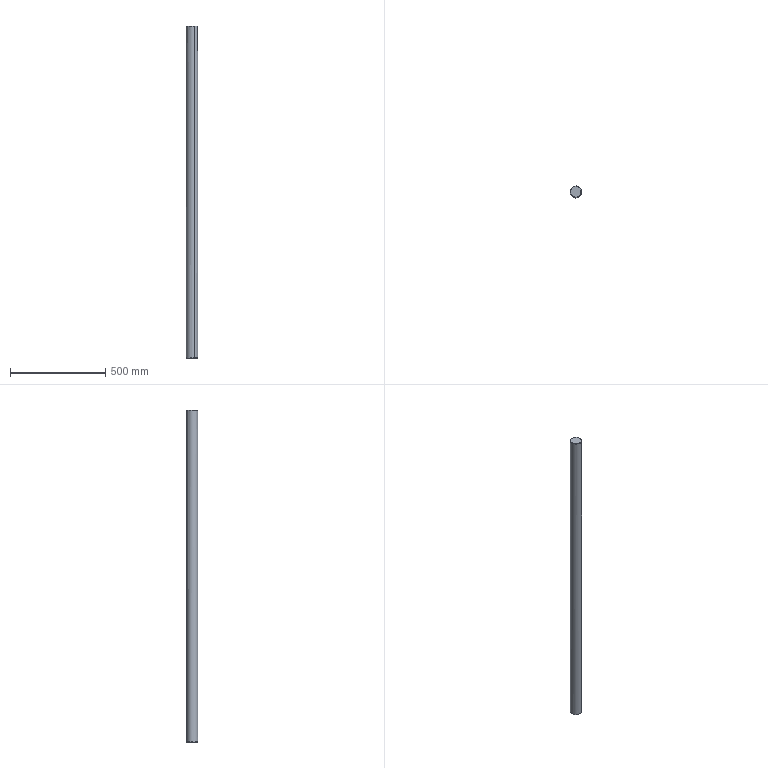Part | SolidWorks | features BaseBody 1 | 1 solid | 16 faces | box 60 x 60 x 1739 mm | volume 4902443 mm3 | cone 6 | plane 5 | cylinder 5 | commonest cylinder face diameters 18 x3 60 x2
STEP:
#1=CARTESIAN_POINT('',(-163.923,853.249,-864.893));
#2=VERTEX_POINT('',#1);
#3=CARTESIAN_POINT('',(-161.923,853.249,-862.893));
#4=VERTEX_POINT('',#3);
#5=CARTESIAN_POINT('',(-161.923,853.249,-862.893));
#6=DIRECTION('',(0.7071,0.,0.7071));
#7=VECTOR('',#6,1000.);
#8=LINE('',#5,#7);
#9=EDGE_CURVE('',#2,#4,#8,.T.);
#10=ORIENTED_EDGE('',*,*,#9,.F.);
#11=CARTESIAN_POINT('',(-203.98,878.52,-864.893));
#12=VERTEX_POINT('',#11);
#13=CARTESIAN_POINT('',(-191.923,853.249,-864.893));
#14=DIRECTION('',(0.,0.,-1.));
#15=DIRECTION('',(-1.,0.,0.));
#16=AXIS2_PLACEMENT_3D('',#13,#14,#15);
#17=CIRCLE('',#16,28.);
#18=EDGE_CURVE('',#12,#2,#17,.T.);
#19=ORIENTED_EDGE('',*,*,#18,.F.);
#20=CARTESIAN_POINT('',(-204.841,880.325,-862.893));
#21=VERTEX_POINT('',#20);
#22=CARTESIAN_POINT('',(-203.98,878.52,-864.893));
#23=DIRECTION('',(-0.3045,0.6382,0.7071));
#24=VECTOR('',#23,1000.);
#25=LINE('',#22,#24);
#26=EDGE_CURVE('',#12,#21,#25,.T.);
#27=ORIENTED_EDGE('',*,*,#26,.T.);
#28=CARTESIAN_POINT('',(-191.923,853.249,-862.893));
#29=DIRECTION('',(0.,0.,1.));
#30=DIRECTION('',(-1.,0.,0.));
#31=AXIS2_PLACEMENT_3D('',#28,#29,#30);
#32=CIRCLE('',#31,30.);
#33=EDGE_CURVE('',#4,#21,#32,.T.);
#34=ORIENTED_EDGE('',*,*,#33,.F.);
#35=EDGE_LOOP('',(#10,#19,#27,#34));
#36=FACE_OUTER_BOUND('',#35,.T.);
#37=CARTESIAN_POINT('',(-191.923,853.249,-862.893));
#38=DIRECTION('',(0.,0.,1.));
#39=DIRECTION('',(1.,0.,0.));
#40=AXIS2_PLACEMENT_3D('',#37,#38,#39);
#41=CONICAL_SURFACE('',#40,30.,0.7854);
#42=ADVANCED_FACE('',(#36),#41,.T.);
#43=ORIENTED_EDGE('',*,*,#26,.F.);
#44=CARTESIAN_POINT('',(-179.866,827.978,-864.893));
#45=VERTEX_POINT('',#44);
#46=CARTESIAN_POINT('',(-191.923,853.249,-864.893));
#47=DIRECTION('',(0.,0.,-1.));
#48=DIRECTION('',(-1.,0.,0.));
#49=AXIS2_PLACEMENT_3D('',#46,#47,#48);
#50=CIRCLE('',#49,28.);
#51=EDGE_CURVE('',#45,#12,#50,.T.);
#52=ORIENTED_EDGE('',*,*,#51,.F.);
#53=CARTESIAN_POINT('',(-179.005,826.173,-862.893));
#54=VERTEX_POINT('',#53);
#55=CARTESIAN_POINT('',(-179.005,826.173,-862.893));
#56=DIRECTION('',(-0.3045,0.6382,-0.7071));
#57=VECTOR('',#56,1000.);
#58=LINE('',#55,#57);
#59=EDGE_CURVE('',#54,#45,#58,.T.);
#60=ORIENTED_EDGE('',*,*,#59,.F.);
#61=CARTESIAN_POINT('',(-191.923,853.249,-862.893));
#62=DIRECTION('',(0.,0.,1.));
#63=DIRECTION('',(-1.,0.,0.));
#64=AXIS2_PLACEMENT_3D('',#61,#62,#63);
#65=CIRCLE('',#64,30.);
#66=EDGE_CURVE('',#21,#54,#65,.T.);
#67=ORIENTED_EDGE('',*,*,#66,.F.);
#68=EDGE_LOOP('',(#43,#52,#60,#67));
#69=FACE_OUTER_BOUND('',#68,.T.);
#70=CARTESIAN_POINT('',(-191.923,853.249,-862.893));
#71=DIRECTION('',(0.,0.,1.));
#72=DIRECTION('',(1.,0.,0.));
#73=AXIS2_PLACEMENT_3D('',#70,#71,#72);
#74=CONICAL_SURFACE('',#73,30.,0.7854);
#75=ADVANCED_FACE('',(#69),#74,.T.);
#76=ORIENTED_EDGE('',*,*,#51,.T.);
#77=ORIENTED_EDGE('',*,*,#18,.T.);
#78=CARTESIAN_POINT('',(-191.923,853.249,-864.893));
#79=DIRECTION('',(0.,0.,-1.));
#80=DIRECTION('',(-1.,0.,0.));
#81=AXIS2_PLACEMENT_3D('',#78,#79,#80);
#82=CIRCLE('',#81,28.);
#83=EDGE_CURVE('',#2,#45,#82,.T.);
#84=ORIENTED_EDGE('',*,*,#83,.T.);
#85=EDGE_LOOP('',(#76,#77,#84));
#86=FACE_OUTER_BOUND('',#85,.T.);
#87=CARTESIAN_POINT('',(-191.923,853.249,-864.893));
#88=DIRECTION('',(0.,0.,-1.));
#89=DIRECTION('',(0.,-1.,0.));
#90=AXIS2_PLACEMENT_3D('',#87,#88,#89);
#91=PLANE('',#90);
#92=ADVANCED_FACE('',(#86),#91,.T.);
#93=CARTESIAN_POINT('',(-204.841,880.325,872.033));
#94=VERTEX_POINT('',#93);
#95=CARTESIAN_POINT('',(-204.841,880.325,-50.893));
#96=DIRECTION('',(0.,0.,1.));
#97=VECTOR('',#96,1000.);
#98=LINE('',#95,#97);
#99=EDGE_CURVE('',#21,#94,#98,.T.);
#100=ORIENTED_EDGE('',*,*,#99,.F.);
#101=ORIENTED_EDGE('',*,*,#66,.T.);
#102=CARTESIAN_POINT('',(-179.005,826.173,872.033));
#103=VERTEX_POINT('',#102);
#104=CARTESIAN_POINT('',(-179.005,826.173,-50.893));
#105=DIRECTION('',(0.,0.,1.));
#106=VECTOR('',#105,1000.);
#107=LINE('',#104,#106);
#108=EDGE_CURVE('',#54,#103,#107,.T.);
#109=ORIENTED_EDGE('',*,*,#108,.T.);
#110=CARTESIAN_POINT('',(-221.923,853.249,872.033));
#111=VERTEX_POINT('',#110);
#112=CARTESIAN_POINT('',(-191.923,853.249,872.033));
#113=DIRECTION('',(0.,0.,-1.));
#114=DIRECTION('',(-1.,0.,0.));
#115=AXIS2_PLACEMENT_3D('',#112,#113,#114);
#116=CIRCLE('',#115,30.);
#117=EDGE_CURVE('',#103,#111,#116,.T.);
#118=ORIENTED_EDGE('',*,*,#117,.T.);
#119=CARTESIAN_POINT('',(-191.923,853.249,872.033));
#120=DIRECTION('',(0.,0.,-1.));
#121=DIRECTION('',(-1.,0.,0.));
#122=AXIS2_PLACEMENT_3D('',#119,#120,#121);
#123=CIRCLE('',#122,30.);
#124=EDGE_CURVE('',#111,#94,#123,.T.);
#125=ORIENTED_EDGE('',*,*,#124,.T.);
#126=EDGE_LOOP('',(#100,#101,#109,#118,#125));
#127=FACE_OUTER_BOUND('',#126,.T.);
#128=CARTESIAN_POINT('',(-191.923,853.249,-50.893));
#129=DIRECTION('',(0.,0.,1.));
#130=DIRECTION('',(0.4306,-0.9025,0.));
#131=AXIS2_PLACEMENT_3D('',#128,#129,#130);
#132=CYLINDRICAL_SURFACE('',#131,30.);
#133=ADVANCED_FACE('',(#127),#132,.T.);
#134=CARTESIAN_POINT('',(-163.305,844.249,749.107));
#135=VERTEX_POINT('',#134);
#136=CARTESIAN_POINT('',(-161.923,853.249,740.107));
#137=VERTEX_POINT('',#136);
#138=CARTESIAN_POINT('',(-163.305,844.249,749.107));
#139=CARTESIAN_POINT('',(-163.305,844.249,748.815));
#140=CARTESIAN_POINT('',(-163.3,844.263,748.521));
#141=CARTESIAN_POINT('',(-163.287,844.307,748.079));
#142=CARTESIAN_POINT('',(-163.278,844.334,747.858));
#143=CARTESIAN_POINT('',(-163.265,844.375,747.6));
#144=CARTESIAN_POINT('',(-163.258,844.399,747.471));
#145=CARTESIAN_POINT('',(-163.255,844.409,747.416));
#146=CARTESIAN_POINT('',(-163.253,844.416,747.379));
#147=CARTESIAN_POINT('',(-163.252,844.42,747.36));
#148=CARTESIAN_POINT('',(-163.234,844.479,747.066));
#149=CARTESIAN_POINT('',(-163.212,844.548,746.786));
#150=CARTESIAN_POINT('',(-163.174,844.677,746.361));
#151=CARTESIAN_POINT('',(-163.16,844.724,746.219));
#152=CARTESIAN_POINT('',(-163.137,844.8,746.005));
#153=CARTESIAN_POINT('',(-163.126,844.84,745.898));
#154=CARTESIAN_POINT('',(-163.111,844.889,745.772));
#155=CARTESIAN_POINT('',(-163.104,844.915,745.71));
#156=CARTESIAN_POINT('',(-163.101,844.926,745.683));
#157=CARTESIAN_POINT('',(-163.099,844.933,745.665));
#158=CARTESIAN_POINT('',(-163.098,844.937,745.655));
#159=CARTESIAN_POINT('',(-163.068,845.041,745.405));
#160=CARTESIAN_POINT('',(-163.034,845.159,745.153));
#161=CARTESIAN_POINT('',(-162.978,845.364,744.764));
#162=CARTESIAN_POINT('',(-162.958,845.438,744.633));
#163=CARTESIAN_POINT('',(-162.926,845.556,744.434));
#164=CARTESIAN_POINT('',(-162.91,845.618,744.334));
#165=CARTESIAN_POINT('',(-162.89,845.693,744.217));
#166=CARTESIAN_POINT('',(-162.88,845.731,744.158));
#167=CARTESIAN_POINT('',(-162.875,845.751,744.129));
#168=CARTESIAN_POINT('',(-162.873,845.759,744.116));
#169=CARTESIAN_POINT('',(-162.872,845.765,744.108));
#170=CARTESIAN_POINT('',(-162.871,845.769,744.102));
#171=CARTESIAN_POINT('',(-162.844,845.872,743.948));
#172=CARTESIAN_POINT('',(-162.809,846.009,743.753));
#173=CARTESIAN_POINT('',(-162.743,846.282,743.407));
#174=CARTESIAN_POINT('',(-162.718,846.385,743.283));
#175=CARTESIAN_POINT('',(-162.679,846.558,743.087));
#176=CARTESIAN_POINT('',(-162.665,846.619,743.02));
#177=CARTESIAN_POINT('',(-162.643,846.716,742.916));
#178=CARTESIAN_POINT('',(-162.632,846.765,742.864));
#179=CARTESIAN_POINT('',(-162.621,846.817,742.811));
#180=CARTESIAN_POINT('',(-162.613,846.852,742.776));
#181=CARTESIAN_POINT('',(-162.609,846.871,742.757));
#182=CARTESIAN_POINT('',(-162.547,847.155,742.473));
#183=CARTESIAN_POINT('',(-162.496,847.409,742.253));
#184=CARTESIAN_POINT('',(-162.431,847.752,741.979));
#185=CARTESIAN_POINT('',(-162.411,847.86,741.897));
#186=CARTESIAN_POINT('',(-162.384,848.012,741.787));
#187=CARTESIAN_POINT('',(-162.375,848.061,741.752));
#188=CARTESIAN_POINT('',(-162.363,848.132,741.703));
#189=CARTESIAN_POINT('',(-162.357,848.166,741.679));
#190=CARTESIAN_POINT('',(-162.35,848.205,741.653));
#191=CARTESIAN_POINT('',(-162.347,848.224,741.64));
#192=CARTESIAN_POINT('',(-162.345,848.233,741.634));
#193=CARTESIAN_POINT('',(-162.345,848.238,741.631));
#194=CARTESIAN_POINT('',(-162.344,848.239,741.63));
#195=CARTESIAN_POINT('',(-162.299,848.51,741.449));
#196=CARTESIAN_POINT('',(-162.258,848.775,741.292));
#197=CARTESIAN_POINT('',(-162.202,849.164,741.086));
#198=CARTESIAN_POINT('',(-162.185,849.293,741.022));
#199=CARTESIAN_POINT('',(-162.16,849.483,740.932));
#200=CARTESIAN_POINT('',(-162.149,849.577,740.889));
#201=CARTESIAN_POINT('',(-162.135,849.687,740.842));
#202=CARTESIAN_POINT('',(-162.129,849.741,740.819));
#203=CARTESIAN_POINT('',(-162.126,849.764,740.809));
#204=CARTESIAN_POINT('',(-162.124,849.779,740.802));
#205=CARTESIAN_POINT('',(-162.124,849.786,740.8));
#206=CARTESIAN_POINT('',(-162.09,850.079,740.678));
#207=CARTESIAN_POINT('',(-162.061,850.364,740.577));
#208=CARTESIAN_POINT('',(-162.024,850.788,740.448));
#209=CARTESIAN_POINT('',(-162.013,850.929,740.41));
#210=CARTESIAN_POINT('',(-161.997,851.14,740.357));
#211=CARTESIAN_POINT('',(-161.99,851.245,740.332));
#212=CARTESIAN_POINT('',(-161.983,851.35,740.309));
#213=CARTESIAN_POINT('',(-161.979,851.42,740.294));
#214=CARTESIAN_POINT('',(-161.977,851.453,740.288));
#215=CARTESIAN_POINT('',(-161.94,852.075,740.164));
#216=CARTESIAN_POINT('',(-161.923,852.666,740.107));
#217=CARTESIAN_POINT('',(-161.923,853.249,740.107));
#218=B_SPLINE_CURVE_WITH_KNOTS('',3,(#138,#139,#140,#141,#142,#143,#144,#145,#146,#147,#148,#149,#150,#151,#152,#153,#154,#155,#156,#157,#158,#159,#160,#161,#162,#163,#164,#165,#166,#167,#168,#169,#170,#171,#172,#173,#174,#175,#176,#177,#178,#179,#180,#181,#182,#183,#184,#185,#186,#187,#188,#189,#190,#191,#192,#193,#194,#195,#196,#197,#198,#199,#200,#201,#202,#203,#204,#205,#206,#207,#208,#209,#210,#211,#212,#213,#214,#215,#216,#217),.UNSPECIFIED.,.F.,.F.,(4,2,1,1,1,2,2,2,2,1,1,1,2,2,2,2,1,1,1,1,2,2,2,2,2,1,2,2,2,2,2,1,1,1,2,2,2,2,1,1,1,2,2,2,2,1,2,2,4),(0.,0.0625,0.09375,0.1094,0.1172,0.1211,0.125,0.1875,0.2187,0.2344,0.2422,0.2461,0.248,0.25,0.3125,0.3437,0.3594,0.3672,0.3711,0.373,0.374,0.375,0.4375,0.4687,0.4844,0.4922,0.4961,0.5,0.5625,0.5937,0.6094,0.6172,0.6211,0.623,0.624,0.625,0.6875,0.7187,0.7344,0.7422,0.7461,0.748,0.75,0.8125,0.8437,0.8594,0.8672,0.875,1.),.UNSPECIFIED.);
#219=EDGE_CURVE('',#135,#137,#218,.T.);
#220=ORIENTED_EDGE('',*,*,#219,.F.);
#221=CARTESIAN_POINT('',(-163.305,844.249,861.107));
#222=VERTEX_POINT('',#221);
#223=CARTESIAN_POINT('',(-163.305,844.249,-50.893));
#224=DIRECTION('',(0.,0.,1.));
#225=VECTOR('',#224,1000.);
#226=LINE('',#223,#225);
#227=EDGE_CURVE('',#135,#222,#226,.T.);
#228=ORIENTED_EDGE('',*,*,#227,.T.);
#229=CARTESIAN_POINT('',(-163.305,862.249,861.107));
#230=VERTEX_POINT('',#229);
#231=CARTESIAN_POINT('',(-163.305,862.249,861.107));
#232=CARTESIAN_POINT('',(-163.305,862.249,861.398));
#233=CARTESIAN_POINT('',(-163.3,862.235,861.692));
#234=CARTESIAN_POINT('',(-163.287,862.191,862.133));
#235=CARTESIAN_POINT('',(-163.278,862.164,862.354));
#236=CARTESIAN_POINT('',(-163.266,862.123,862.612));
#237=CARTESIAN_POINT('',(-163.258,862.099,862.741));
#238=CARTESIAN_POINT('',(-163.255,862.089,862.796));
#239=CARTESIAN_POINT('',(-163.253,862.082,862.833));
#240=CARTESIAN_POINT('',(-163.252,862.078,862.852));
#241=CARTESIAN_POINT('',(-163.234,862.019,863.146));
#242=CARTESIAN_POINT('',(-163.212,861.95,863.426));
#243=CARTESIAN_POINT('',(-163.174,861.822,863.851));
#244=CARTESIAN_POINT('',(-163.16,861.775,863.993));
#245=CARTESIAN_POINT('',(-163.138,861.698,864.207));
#246=CARTESIAN_POINT('',(-163.126,861.659,864.314));
#247=CARTESIAN_POINT('',(-163.112,861.609,864.439));
#248=CARTESIAN_POINT('',(-163.104,861.584,864.502));
#249=CARTESIAN_POINT('',(-163.101,861.573,864.528));
#250=CARTESIAN_POINT('',(-163.099,861.566,864.546));
#251=CARTESIAN_POINT('',(-163.098,861.562,864.557));
#252=CARTESIAN_POINT('',(-163.068,861.458,864.806));
#253=CARTESIAN_POINT('',(-163.034,861.34,865.058));
#254=CARTESIAN_POINT('',(-162.978,861.135,865.447));
#255=CARTESIAN_POINT('',(-162.958,861.061,865.578));
#256=CARTESIAN_POINT('',(-162.926,860.943,865.777));
#257=CARTESIAN_POINT('',(-162.91,860.882,865.876));
#258=CARTESIAN_POINT('',(-162.891,860.807,865.994));
#259=CARTESIAN_POINT('',(-162.881,860.768,866.052));
#260=CARTESIAN_POINT('',(-162.876,860.749,866.082));
#261=CARTESIAN_POINT('',(-162.874,860.741,866.094));
#262=CARTESIAN_POINT('',(-162.872,860.735,866.103));
#263=CARTESIAN_POINT('',(-162.871,860.731,866.109));
#264=CARTESIAN_POINT('',(-162.844,860.628,866.263));
#265=CARTESIAN_POINT('',(-162.809,860.491,866.458));
#266=CARTESIAN_POINT('',(-162.743,860.218,866.804));
#267=CARTESIAN_POINT('',(-162.719,860.115,866.928));
#268=CARTESIAN_POINT('',(-162.679,859.942,867.124));
#269=CARTESIAN_POINT('',(-162.665,859.881,867.191));
#270=CARTESIAN_POINT('',(-162.644,859.785,867.294));
#271=CARTESIAN_POINT('',(-162.633,859.735,867.346));
#272=CARTESIAN_POINT('',(-162.621,859.684,867.399));
#273=CARTESIAN_POINT('',(-162.614,859.649,867.435));
#274=CARTESIAN_POINT('',(-162.61,859.63,867.454));
#275=CARTESIAN_POINT('',(-162.548,859.346,867.738));
#276=CARTESIAN_POINT('',(-162.497,859.092,867.958));
#277=CARTESIAN_POINT('',(-162.432,858.749,868.232));
#278=CARTESIAN_POINT('',(-162.412,858.641,868.314));
#279=CARTESIAN_POINT('',(-162.384,858.49,868.424));
#280=CARTESIAN_POINT('',(-162.376,858.441,868.458));
#281=CARTESIAN_POINT('',(-162.364,858.371,868.507));
#282=CARTESIAN_POINT('',(-162.358,858.336,868.531));
#283=CARTESIAN_POINT('',(-162.351,858.297,868.558));
#284=CARTESIAN_POINT('',(-162.348,858.278,868.57));
#285=CARTESIAN_POINT('',(-162.346,858.27,868.576));
#286=CARTESIAN_POINT('',(-162.345,858.264,868.58));
#287=CARTESIAN_POINT('',(-162.345,858.263,868.58));
#288=CARTESIAN_POINT('',(-162.299,857.993,868.762));
#289=CARTESIAN_POINT('',(-162.258,857.728,868.918));
#290=CARTESIAN_POINT('',(-162.203,857.339,869.125));
#291=CARTESIAN_POINT('',(-162.186,857.211,869.189));
#292=CARTESIAN_POINT('',(-162.161,857.021,869.279));
#293=CARTESIAN_POINT('',(-162.149,856.926,869.322));
#294=CARTESIAN_POINT('',(-162.136,856.817,869.369));
#295=CARTESIAN_POINT('',(-162.13,856.763,869.392));
#296=CARTESIAN_POINT('',(-162.127,856.74,869.402));
#297=CARTESIAN_POINT('',(-162.125,856.725,869.408));
#298=CARTESIAN_POINT('',(-162.124,856.718,869.411));
#299=CARTESIAN_POINT('',(-162.09,856.425,869.533));
#300=CARTESIAN_POINT('',(-162.062,856.141,869.635));
#301=CARTESIAN_POINT('',(-162.024,855.717,869.763));
#302=CARTESIAN_POINT('',(-162.013,855.576,869.802));
#303=CARTESIAN_POINT('',(-161.998,855.365,869.855));
#304=CARTESIAN_POINT('',(-161.99,855.26,869.88));
#305=CARTESIAN_POINT('',(-161.984,855.155,869.903));
#306=CARTESIAN_POINT('',(-161.979,855.086,869.917));
#307=CARTESIAN_POINT('',(-161.977,855.053,869.924));
#308=CARTESIAN_POINT('',(-161.958,854.723,869.99));
#309=CARTESIAN_POINT('',(-161.945,854.43,870.034));
#310=CARTESIAN_POINT('',(-161.928,853.842,870.092));
#311=CARTESIAN_POINT('',(-161.923,853.551,870.106));
#312=CARTESIAN_POINT('',(-161.923,852.965,870.107));
#313=CARTESIAN_POINT('',(-161.927,852.67,870.093));
#314=CARTESIAN_POINT('',(-161.94,852.227,870.05));
#315=CARTESIAN_POINT('',(-161.948,852.005,870.022));
#316=CARTESIAN_POINT('',(-161.961,851.746,869.981));
#317=CARTESIAN_POINT('',(-161.967,851.617,869.958));
#318=CARTESIAN_POINT('',(-161.971,851.562,869.947));
#319=CARTESIAN_POINT('',(-161.973,851.525,869.94));
#320=CARTESIAN_POINT('',(-161.974,851.506,869.936));
#321=CARTESIAN_POINT('',(-161.991,851.211,869.878));
#322=CARTESIAN_POINT('',(-162.012,850.931,869.808));
#323=CARTESIAN_POINT('',(-162.048,850.508,869.68));
#324=CARTESIAN_POINT('',(-162.062,850.367,869.634));
#325=CARTESIAN_POINT('',(-162.083,850.154,869.558));
#326=CARTESIAN_POINT('',(-162.094,850.048,869.519));
#327=CARTESIAN_POINT('',(-162.108,849.924,869.47));
#328=CARTESIAN_POINT('',(-162.115,849.862,869.445));
#329=CARTESIAN_POINT('',(-162.118,849.835,869.434));
#330=CARTESIAN_POINT('',(-162.12,849.818,869.427));
#331=CARTESIAN_POINT('',(-162.121,849.808,869.423));
#332=CARTESIAN_POINT('',(-162.151,849.553,869.317));
#333=CARTESIAN_POINT('',(-162.183,849.298,869.199));
#334=CARTESIAN_POINT('',(-162.239,848.908,868.992));
#335=CARTESIAN_POINT('',(-162.258,848.777,868.919));
#336=CARTESIAN_POINT('',(-162.289,848.579,868.801));
#337=CARTESIAN_POINT('',(-162.305,848.479,868.74));
#338=CARTESIAN_POINT('',(-162.324,848.363,868.665));
#339=CARTESIAN_POINT('',(-162.333,848.304,868.627));
#340=CARTESIAN_POINT('',(-162.338,848.275,868.608));
#341=CARTESIAN_POINT('',(-162.34,848.263,868.599));
#342=CARTESIAN_POINT('',(-162.342,848.254,868.594));
#343=CARTESIAN_POINT('',(-162.343,848.249,868.59));
#344=CARTESIAN_POINT('',(-162.372,848.073,868.472));
#345=CARTESIAN_POINT('',(-162.409,847.868,868.327));
#346=CARTESIAN_POINT('',(-162.474,847.524,868.053));
#347=CARTESIAN_POINT('',(-162.498,847.403,867.952));
#348=CARTESIAN_POINT('',(-162.536,847.215,867.784));
#349=CARTESIAN_POINT('',(-162.55,847.15,867.726));
#350=CARTESIAN_POINT('',(-162.57,847.053,867.634));
#351=CARTESIAN_POINT('',(-162.58,847.004,867.587));
#352=CARTESIAN_POINT('',(-162.591,846.954,867.539));
#353=CARTESIAN_POINT('',(-162.598,846.92,867.506));
#354=CARTESIAN_POINT('',(-162.602,846.905,867.49));
#355=CARTESIAN_POINT('',(-162.667,846.602,867.188));
#356=CARTESIAN_POINT('',(-162.72,846.375,866.924));
#357=CARTESIAN_POINT('',(-162.786,846.103,866.58));
#358=CARTESIAN_POINT('',(-162.806,846.024,866.475));
#359=CARTESIAN_POINT('',(-162.832,845.92,866.331));
#360=CARTESIAN_POINT('',(-162.84,845.888,866.285));
#361=CARTESIAN_POINT('',(-162.852,845.843,866.221));
#362=CARTESIAN_POINT('',(-162.857,845.822,866.19));
#363=CARTESIAN_POINT('',(-162.863,845.798,866.155));
#364=CARTESIAN_POINT('',(-162.866,845.787,866.138));
#365=CARTESIAN_POINT('',(-162.867,845.781,866.13));
#366=CARTESIAN_POINT('',(-162.868,845.779,866.126));
#367=CARTESIAN_POINT('',(-162.868,845.777,866.124));
#368=CARTESIAN_POINT('',(-162.869,845.777,866.124));
#369=CARTESIAN_POINT('',(-162.916,845.594,865.851));
#370=CARTESIAN_POINT('',(-162.958,845.436,865.584));
#371=CARTESIAN_POINT('',(-163.015,845.229,865.194));
#372=CARTESIAN_POINT('',(-163.033,845.165,865.065));
#373=CARTESIAN_POINT('',(-163.058,845.076,864.876));
#374=CARTESIAN_POINT('',(-163.07,845.033,864.782));
#375=CARTESIAN_POINT('',(-163.083,844.986,864.674));
#376=CARTESIAN_POINT('',(-163.09,844.963,864.621));
#377=CARTESIAN_POINT('',(-163.093,844.954,864.598));
#378=CARTESIAN_POINT('',(-163.095,844.947,864.583));
#379=CARTESIAN_POINT('',(-163.095,844.945,864.576));
#380=CARTESIAN_POINT('',(-163.131,844.823,864.283));
#381=CARTESIAN_POINT('',(-163.16,844.721,864.));
#382=CARTESIAN_POINT('',(-163.199,844.594,863.578));
#383=CARTESIAN_POINT('',(-163.21,844.555,863.438));
#384=CARTESIAN_POINT('',(-163.226,844.502,863.229));
#385=CARTESIAN_POINT('',(-163.234,844.478,863.125));
#386=CARTESIAN_POINT('',(-163.242,844.451,863.004));
#387=CARTESIAN_POINT('',(-163.245,844.44,862.953));
#388=CARTESIAN_POINT('',(-163.248,844.433,862.918));
#389=CARTESIAN_POINT('',(-163.249,844.43,862.902));
#390=CARTESIAN_POINT('',(-163.287,844.307,862.291));
#391=CARTESIAN_POINT('',(-163.305,844.249,861.694));
#392=CARTESIAN_POINT('',(-163.305,844.249,861.107));
#393=B_SPLINE_CURVE_WITH_KNOTS('',3,(#231,#232,#233,#234,#235,#236,#237,#238,#239,#240,#241,#242,#243,#244,#245,#246,#247,#248,#249,#250,#251,#252,#253,#254,#255,#256,#257,#258,#259,#260,#261,#262,#263,#264,#265,#266,#267,#268,#269,#270,#271,#272,#273,#274,#275,#276,#277,#278,#279,#280,#281,#282,#283,#284,#285,#286,#287,#288,#289,#290,#291,#292,#293,#294,#295,#296,#297,#298,#299,#300,#301,#302,#303,#304,#305,#306,#307,#308,#309,#310,#311,#312,#313,#314,#315,#316,#317,#318,#319,#320,#321,#322,#323,#324,#325,#326,#327,#328,#329,#330,#331,#332,#333,#334,#335,#336,#337,#338,#339,#340,#341,#342,#343,#344,#345,#346,#347,#348,#349,#350,#351,#352,#353,#354,#355,#356,#357,#358,#359,#360,#361,#362,#363,#364,#365,#366,#367,#368,#369,#370,#371,#372,#373,#374,#375,#376,#377,#378,#379,#380,#381,#382,#383,#384,#385,#386,#387,#388,#389,#390,#391,#392),.UNSPECIFIED.,.F.,.F.,(4,2,1,1,1,2,2,2,2,1,1,1,2,2,2,2,1,1,1,1,2,2,2,2,2,1,2,2,2,2,2,1,1,1,2,2,2,2,1,1,1,2,2,2,2,1,2,2,2,2,2,1,1,1,2,2,2,2,1,1,1,2,2,2,2,1,1,1,1,2,2,2,2,2,1,2,2,2,2,2,1,1,1,1,2,2,2,2,1,1,1,2,2,2,2,1,1,2,2,4),(0.,0.03125,0.04687,0.05469,0.05859,0.06055,0.0625,0.09375,0.1094,0.1172,0.1211,0.123,0.124,0.125,0.1562,0.1719,0.1797,0.1836,0.1855,0.1865,0.187,0.1875,0.2187,0.2344,0.2422,0.2461,0.248,0.25,0.2812,0.2969,0.3047,0.3086,0.3105,0.3115,0.312,0.3125,0.3437,0.3594,0.3672,0.3711,0.373,0.374,0.375,0.4062,0.4219,0.4297,0.4336,0.4375,0.4687,0.5,0.5312,0.5469,0.5547,0.5586,0.5605,0.5625,0.5937,0.6094,0.6172,0.6211,0.623,0.624,0.625,0.6562,0.6719,0.6797,0.6836,0.6855,0.6865,0.687,0.6875,0.7187,0.7344,0.7422,0.7461,0.748,0.75,0.7812,0.7969,0.8047,0.8086,0.8105,0.8115,0.812,0.8123,0.8125,0.8437,0.8594,0.8672,0.8711,0.873,0.874,0.875,0.9062,0.9219,0.9297,0.9336,0.9355,0.9375,1.),.UNSPECIFIED.);
#394=EDGE_CURVE('',#230,#222,#393,.T.);
#395=ORIENTED_EDGE('',*,*,#394,.F.);
#396=CARTESIAN_POINT('',(-163.305,862.249,749.107));
#397=VERTEX_POINT('',#396);
#398=CARTESIAN_POINT('',(-163.305,862.249,-50.893));
#399=DIRECTION('',(0.,0.,-1.));
#400=VECTOR('',#399,1000.);
#401=LINE('',#398,#400);
#402=EDGE_CURVE('',#230,#397,#401,.T.);
#403=ORIENTED_EDGE('',*,*,#402,.T.);
#404=CARTESIAN_POINT('',(-161.923,853.249,740.107));
#405=CARTESIAN_POINT('',(-161.923,853.542,740.107));
#406=CARTESIAN_POINT('',(-161.927,853.837,740.121));
#407=CARTESIAN_POINT('',(-161.94,854.279,740.165));
#408=CARTESIAN_POINT('',(-161.949,854.501,740.192));
#409=CARTESIAN_POINT('',(-161.961,854.759,740.234));
#410=CARTESIAN_POINT('',(-161.968,854.888,740.257));
#411=CARTESIAN_POINT('',(-161.971,854.943,740.268));
#412=CARTESIAN_POINT('',(-161.973,854.98,740.275));
#413=CARTESIAN_POINT('',(-161.974,855.,740.279));
#414=CARTESIAN_POINT('',(-161.992,855.294,740.338));
#415=CARTESIAN_POINT('',(-162.012,855.574,740.407));
#416=CARTESIAN_POINT('',(-162.049,855.997,740.535));
#417=CARTESIAN_POINT('',(-162.062,856.138,740.582));
#418=CARTESIAN_POINT('',(-162.084,856.35,740.658));
#419=CARTESIAN_POINT('',(-162.095,856.456,740.697));
#420=CARTESIAN_POINT('',(-162.109,856.58,740.746));
#421=CARTESIAN_POINT('',(-162.116,856.642,740.771));
#422=CARTESIAN_POINT('',(-162.119,856.669,740.782));
#423=CARTESIAN_POINT('',(-162.121,856.686,740.789));
#424=CARTESIAN_POINT('',(-162.122,856.696,740.793));
#425=CARTESIAN_POINT('',(-162.151,856.951,740.899));
#426=CARTESIAN_POINT('',(-162.184,857.205,741.017));
#427=CARTESIAN_POINT('',(-162.239,857.595,741.224));
#428=CARTESIAN_POINT('',(-162.259,857.726,741.298));
#429=CARTESIAN_POINT('',(-162.29,857.924,741.416));
#430=CARTESIAN_POINT('',(-162.305,858.023,741.477));
#431=CARTESIAN_POINT('',(-162.324,858.14,741.551));
#432=CARTESIAN_POINT('',(-162.334,858.198,741.59));
#433=CARTESIAN_POINT('',(-162.339,858.227,741.609));
#434=CARTESIAN_POINT('',(-162.341,858.24,741.617));
#435=CARTESIAN_POINT('',(-162.343,858.248,741.623));
#436=CARTESIAN_POINT('',(-162.344,858.254,741.627));
#437=CARTESIAN_POINT('',(-162.373,858.429,741.744));
#438=CARTESIAN_POINT('',(-162.41,858.633,741.889));
#439=CARTESIAN_POINT('',(-162.475,858.977,742.163));
#440=CARTESIAN_POINT('',(-162.499,859.098,742.264));
#441=CARTESIAN_POINT('',(-162.537,859.287,742.432));
#442=CARTESIAN_POINT('',(-162.55,859.351,742.49));
#443=CARTESIAN_POINT('',(-162.571,859.448,742.582));
#444=CARTESIAN_POINT('',(-162.581,859.498,742.629));
#445=CARTESIAN_POINT('',(-162.592,859.547,742.678));
#446=CARTESIAN_POINT('',(-162.599,859.581,742.711));
#447=CARTESIAN_POINT('',(-162.602,859.596,742.726));
#448=CARTESIAN_POINT('',(-162.668,859.898,743.028));
#449=CARTESIAN_POINT('',(-162.721,860.124,743.292));
#450=CARTESIAN_POINT('',(-162.786,860.396,743.635));
#451=CARTESIAN_POINT('',(-162.806,860.475,743.741));
#452=CARTESIAN_POINT('',(-162.832,860.579,743.885));
#453=CARTESIAN_POINT('',(-162.841,860.612,743.93));
#454=CARTESIAN_POINT('',(-162.852,860.656,743.995));
#455=CARTESIAN_POINT('',(-162.857,860.678,744.026));
#456=CARTESIAN_POINT('',(-162.864,860.702,744.061));
#457=CARTESIAN_POINT('',(-162.866,860.713,744.078));
#458=CARTESIAN_POINT('',(-162.868,860.719,744.086));
#459=CARTESIAN_POINT('',(-162.869,860.721,744.09));
#460=CARTESIAN_POINT('',(-162.869,860.723,744.092));
#461=CARTESIAN_POINT('',(-162.869,860.723,744.093));
#462=CARTESIAN_POINT('',(-162.916,860.905,744.365));
#463=CARTESIAN_POINT('',(-162.958,861.063,744.632));
#464=CARTESIAN_POINT('',(-163.015,861.27,745.022));
#465=CARTESIAN_POINT('',(-163.033,861.334,745.15));
#466=CARTESIAN_POINT('',(-163.058,861.423,745.34));
#467=CARTESIAN_POINT('',(-163.07,861.466,745.433));
#468=CARTESIAN_POINT('',(-163.084,861.513,745.541));
#469=CARTESIAN_POINT('',(-163.09,861.535,745.595));
#470=CARTESIAN_POINT('',(-163.093,861.545,745.618));
#471=CARTESIAN_POINT('',(-163.095,861.551,745.633));
#472=CARTESIAN_POINT('',(-163.096,861.554,745.639));
#473=CARTESIAN_POINT('',(-163.131,861.676,745.932));
#474=CARTESIAN_POINT('',(-163.161,861.777,746.216));
#475=CARTESIAN_POINT('',(-163.199,861.905,746.637));
#476=CARTESIAN_POINT('',(-163.211,861.943,746.777));
#477=CARTESIAN_POINT('',(-163.226,861.996,746.986));
#478=CARTESIAN_POINT('',(-163.234,862.021,747.09));
#479=CARTESIAN_POINT('',(-163.242,862.047,747.21));
#480=CARTESIAN_POINT('',(-163.246,862.058,747.262));
#481=CARTESIAN_POINT('',(-163.248,862.065,747.296));
#482=CARTESIAN_POINT('',(-163.249,862.068,747.312));
#483=CARTESIAN_POINT('',(-163.287,862.191,747.923));
#484=CARTESIAN_POINT('',(-163.305,862.249,748.519));
#485=CARTESIAN_POINT('',(-163.305,862.249,749.107));
#486=B_SPLINE_CURVE_WITH_KNOTS('',3,(#404,#405,#406,#407,#408,#409,#410,#411,#412,#413,#414,#415,#416,#417,#418,#419,#420,#421,#422,#423,#424,#425,#426,#427,#428,#429,#430,#431,#432,#433,#434,#435,#436,#437,#438,#439,#440,#441,#442,#443,#444,#445,#446,#447,#448,#449,#450,#451,#452,#453,#454,#455,#456,#457,#458,#459,#460,#461,#462,#463,#464,#465,#466,#467,#468,#469,#470,#471,#472,#473,#474,#475,#476,#477,#478,#479,#480,#481,#482,#483,#484,#485),.UNSPECIFIED.,.F.,.F.,(4,2,1,1,1,2,2,2,2,1,1,1,2,2,2,2,1,1,1,1,2,2,2,2,2,1,2,2,2,2,2,1,1,1,1,2,2,2,2,1,1,1,2,2,2,2,1,1,2,2,4),(0.,0.0625,0.09375,0.1094,0.1172,0.1211,0.125,0.1875,0.2188,0.2344,0.2422,0.2461,0.248,0.25,0.3125,0.3438,0.3594,0.3672,0.3711,0.373,0.374,0.375,0.4375,0.4688,0.4844,0.4922,0.4961,0.5,0.5625,0.5938,0.6094,0.6172,0.6211,0.623,0.624,0.6245,0.625,0.6875,0.7188,0.7344,0.7422,0.7461,0.748,0.75,0.8125,0.8438,0.8594,0.8672,0.8711,0.875,1.),.UNSPECIFIED.);
#487=EDGE_CURVE('',#137,#397,#486,.T.);
#488=ORIENTED_EDGE('',*,*,#487,.F.);
#489=EDGE_LOOP('',(#220,#228,#395,#403,#488));
#490=FACE_BOUND('',#489,.T.);
#491=ORIENTED_EDGE('',*,*,#108,.F.);
#492=CARTESIAN_POINT('',(-191.923,853.249,-862.893));
#493=DIRECTION('',(0.,0.,1.));
#494=DIRECTION('',(-1.,0.,0.));
#495=AXIS2_PLACEMENT_3D('',#492,#493,#494);
#496=CIRCLE('',#495,30.);
#497=EDGE_CURVE('',#54,#4,#496,.T.);
#498=ORIENTED_EDGE('',*,*,#497,.T.);
#499=ORIENTED_EDGE('',*,*,#33,.T.);
#500=ORIENTED_EDGE('',*,*,#99,.T.);
#501=CARTESIAN_POINT('',(-191.923,853.249,872.033));
#502=DIRECTION('',(0.,0.,-1.));
#503=DIRECTION('',(-1.,0.,0.));
#504=AXIS2_PLACEMENT_3D('',#501,#502,#503);
#505=CIRCLE('',#504,30.);
#506=EDGE_CURVE('',#94,#103,#505,.T.);
#507=ORIENTED_EDGE('',*,*,#506,.T.);
#508=EDGE_LOOP('',(#491,#498,#499,#500,#507));
#509=FACE_OUTER_BOUND('',#508,.T.);
#510=CARTESIAN_POINT('',(-191.923,853.249,-50.893));
#511=DIRECTION('',(0.,0.,1.));
#512=DIRECTION('',(0.4306,-0.9025,0.));
#513=AXIS2_PLACEMENT_3D('',#510,#511,#512);
#514=CYLINDRICAL_SURFACE('',#513,30.);
#515=ADVANCED_FACE('',(#490,#509),#514,.T.);
#516=CARTESIAN_POINT('',(-168.339,853.249,740.107));
#517=VERTEX_POINT('',#516);
#518=CARTESIAN_POINT('',(-168.339,853.249,740.107));
#519=DIRECTION('',(1.,0.,0.));
#520=VECTOR('',#519,1000.);
#521=LINE('',#518,#520);
#522=EDGE_CURVE('',#517,#137,#521,.T.);
#523=ORIENTED_EDGE('',*,*,#522,.F.);
#524=CARTESIAN_POINT('',(-168.339,844.249,749.107));
#525=VERTEX_POINT('',#524);
#526=CARTESIAN_POINT('',(-168.339,853.249,749.107));
#527=DIRECTION('',(-1.,0.,0.));
#528=DIRECTION('',(0.,0.,1.));
#529=AXIS2_PLACEMENT_3D('',#526,#527,#528);
#530=CIRCLE('',#529,9.);
#531=EDGE_CURVE('',#517,#525,#530,.T.);
#532=ORIENTED_EDGE('',*,*,#531,.T.);
#533=CARTESIAN_POINT('',(-168.339,844.249,749.107));
#534=DIRECTION('',(1.,0.,0.));
#535=VECTOR('',#534,1000.);
#536=LINE('',#533,#535);
#537=EDGE_CURVE('',#525,#135,#536,.T.);
#538=ORIENTED_EDGE('',*,*,#537,.T.);
#539=ORIENTED_EDGE('',*,*,#219,.T.);
#540=EDGE_LOOP('',(#523,#532,#538,#539));
#541=FACE_OUTER_BOUND('',#540,.T.);
#542=CARTESIAN_POINT('',(-168.339,853.249,749.107));
#543=DIRECTION('',(1.,0.,0.));
#544=DIRECTION('',(0.,0.,-1.));
#545=AXIS2_PLACEMENT_3D('',#542,#543,#544);
#546=CYLINDRICAL_SURFACE('',#545,9.);
#547=ADVANCED_FACE('',(#541),#546,.F.);
#548=ORIENTED_EDGE('',*,*,#537,.F.);
#549=CARTESIAN_POINT('',(-168.339,844.249,861.107));
#550=VERTEX_POINT('',#549);
#551=CARTESIAN_POINT('',(-168.339,844.249,681.154));
#552=DIRECTION('',(0.,0.,-1.));
#553=VECTOR('',#552,1000.);
#554=LINE('',#551,#553);
#555=EDGE_CURVE('',#550,#525,#554,.T.);
#556=ORIENTED_EDGE('',*,*,#555,.F.);
#557=CARTESIAN_POINT('',(-168.339,844.249,861.107));
#558=DIRECTION('',(-1.,0.,0.));
#559=VECTOR('',#558,1000.);
#560=LINE('',#557,#559);
#561=EDGE_CURVE('',#222,#550,#560,.T.);
#562=ORIENTED_EDGE('',*,*,#561,.F.);
#563=ORIENTED_EDGE('',*,*,#227,.F.);
#564=EDGE_LOOP('',(#548,#556,#562,#563));
#565=FACE_OUTER_BOUND('',#564,.T.);
#566=CARTESIAN_POINT('',(-168.339,844.249,681.154));
#567=DIRECTION('',(0.,1.,0.));
#568=DIRECTION('',(1.,0.,0.));
#569=AXIS2_PLACEMENT_3D('',#566,#567,#568);
#570=PLANE('',#569);
#571=ADVANCED_FACE('',(#565),#570,.T.);
#572=ORIENTED_EDGE('',*,*,#394,.T.);
#573=ORIENTED_EDGE('',*,*,#561,.T.);
#574=CARTESIAN_POINT('',(-168.339,862.249,861.107));
#575=VERTEX_POINT('',#574);
#576=CARTESIAN_POINT('',(-168.339,853.249,861.107));
#577=DIRECTION('',(-1.,0.,0.));
#578=DIRECTION('',(0.,0.,1.));
#579=AXIS2_PLACEMENT_3D('',#576,#577,#578);
#580=CIRCLE('',#579,9.);
#581=EDGE_CURVE('',#550,#575,#580,.T.);
#582=ORIENTED_EDGE('',*,*,#581,.T.);
#583=CARTESIAN_POINT('',(-168.339,862.249,861.107));
#584=DIRECTION('',(1.,0.,0.));
#585=VECTOR('',#584,1000.);
#586=LINE('',#583,#585);
#587=EDGE_CURVE('',#575,#230,#586,.T.);
#588=ORIENTED_EDGE('',*,*,#587,.T.);
#589=EDGE_LOOP('',(#572,#573,#582,#588));
#590=FACE_OUTER_BOUND('',#589,.T.);
#591=CARTESIAN_POINT('',(-168.339,853.249,861.107));
#592=DIRECTION('',(1.,0.,0.));
#593=DIRECTION('',(0.,0.,-1.));
#594=AXIS2_PLACEMENT_3D('',#591,#592,#593);
#595=CYLINDRICAL_SURFACE('',#594,9.);
#596=ADVANCED_FACE('',(#590),#595,.F.);
#597=ORIENTED_EDGE('',*,*,#587,.F.);
#598=CARTESIAN_POINT('',(-168.339,862.249,749.107));
#599=VERTEX_POINT('',#598);
#600=CARTESIAN_POINT('',(-168.339,862.249,681.154));
#601=DIRECTION('',(0.,0.,1.));
#602=VECTOR('',#601,1000.);
#603=LINE('',#600,#602);
#604=EDGE_CURVE('',#599,#575,#603,.T.);
#605=ORIENTED_EDGE('',*,*,#604,.F.);
#606=CARTESIAN_POINT('',(-168.339,862.249,749.107));
#607=DIRECTION('',(-1.,0.,0.));
#608=VECTOR('',#607,1000.);
#609=LINE('',#606,#608);
#610=EDGE_CURVE('',#397,#599,#609,.T.);
#611=ORIENTED_EDGE('',*,*,#610,.F.);
#612=ORIENTED_EDGE('',*,*,#402,.F.);
#613=EDGE_LOOP('',(#597,#605,#611,#612));
#614=FACE_OUTER_BOUND('',#613,.T.);
#615=CARTESIAN_POINT('',(-168.339,862.249,681.154));
#616=DIRECTION('',(0.,-1.,0.));
#617=DIRECTION('',(0.,0.,-1.));
#618=AXIS2_PLACEMENT_3D('',#615,#616,#617);
#619=PLANE('',#618);
#620=ADVANCED_FACE('',(#614),#619,.T.);
#621=CARTESIAN_POINT('',(-203.98,878.52,874.033));
#622=VERTEX_POINT('',#621);
#623=CARTESIAN_POINT('',(-203.98,878.52,874.033));
#624=DIRECTION('',(-0.3045,0.6382,-0.7071));
#625=VECTOR('',#624,1000.);
#626=LINE('',#623,#625);
#627=EDGE_CURVE('',#622,#94,#626,.T.);
#628=ORIENTED_EDGE('',*,*,#627,.F.);
#629=CARTESIAN_POINT('',(-179.866,827.978,874.033));
#630=VERTEX_POINT('',#629);
#631=CARTESIAN_POINT('',(-191.923,853.249,874.033));
#632=DIRECTION('',(0.,0.,1.));
#633=DIRECTION('',(-1.,0.,0.));
#634=AXIS2_PLACEMENT_3D('',#631,#632,#633);
#635=CIRCLE('',#634,28.);
#636=EDGE_CURVE('',#630,#622,#635,.T.);
#637=ORIENTED_EDGE('',*,*,#636,.F.);
#638=CARTESIAN_POINT('',(-179.005,826.173,872.033));
#639=DIRECTION('',(-0.3045,0.6382,0.7071));
#640=VECTOR('',#639,1000.);
#641=LINE('',#638,#640);
#642=EDGE_CURVE('',#103,#630,#641,.T.);
#643=ORIENTED_EDGE('',*,*,#642,.F.);
#644=ORIENTED_EDGE('',*,*,#506,.F.);
#645=EDGE_LOOP('',(#628,#637,#643,#644));
#646=FACE_OUTER_BOUND('',#645,.T.);
#647=CARTESIAN_POINT('',(-191.923,853.249,872.033));
#648=DIRECTION('',(0.,0.,-1.));
#649=DIRECTION('',(-1.,0.,0.));
#650=AXIS2_PLACEMENT_3D('',#647,#648,#649);
#651=CONICAL_SURFACE('',#650,30.,0.7854);
#652=ADVANCED_FACE('',(#646),#651,.T.);
#653=CARTESIAN_POINT('',(-219.923,853.249,874.033));
#654=VERTEX_POINT('',#653);
#655=CARTESIAN_POINT('',(-221.923,853.249,872.033));
#656=DIRECTION('',(-0.7071,0.,-0.7071));
#657=VECTOR('',#656,1000.);
#658=LINE('',#655,#657);
#659=EDGE_CURVE('',#654,#111,#658,.T.);
#660=ORIENTED_EDGE('',*,*,#659,.F.);
#661=CARTESIAN_POINT('',(-191.923,853.249,874.033));
#662=DIRECTION('',(0.,0.,1.));
#663=DIRECTION('',(-1.,0.,0.));
#664=AXIS2_PLACEMENT_3D('',#661,#662,#663);
#665=CIRCLE('',#664,28.);
#666=EDGE_CURVE('',#622,#654,#665,.T.);
#667=ORIENTED_EDGE('',*,*,#666,.F.);
#668=ORIENTED_EDGE('',*,*,#627,.T.);
#669=ORIENTED_EDGE('',*,*,#124,.F.);
#670=EDGE_LOOP('',(#660,#667,#668,#669));
#671=FACE_OUTER_BOUND('',#670,.T.);
#672=CARTESIAN_POINT('',(-191.923,853.249,872.033));
#673=DIRECTION('',(0.,0.,-1.));
#674=DIRECTION('',(-1.,0.,0.));
#675=AXIS2_PLACEMENT_3D('',#672,#673,#674);
#676=CONICAL_SURFACE('',#675,30.,0.7854);
#677=ADVANCED_FACE('',(#671),#676,.T.);
#678=CARTESIAN_POINT('',(-168.339,853.249,749.107));
#679=DIRECTION('',(-1.,0.,0.));
#680=DIRECTION('',(0.,0.,1.));
#681=AXIS2_PLACEMENT_3D('',#678,#679,#680);
#682=CIRCLE('',#681,9.);
#683=EDGE_CURVE('',#599,#517,#682,.T.);
#684=ORIENTED_EDGE('',*,*,#683,.F.);
#685=ORIENTED_EDGE('',*,*,#604,.T.);
#686=ORIENTED_EDGE('',*,*,#581,.F.);
#687=ORIENTED_EDGE('',*,*,#555,.T.);
#688=ORIENTED_EDGE('',*,*,#531,.F.);
#689=EDGE_LOOP('',(#684,#685,#686,#687,#688));
#690=FACE_OUTER_BOUND('',#689,.T.);
#691=CARTESIAN_POINT('',(-168.339,845.249,681.154));
#692=DIRECTION('',(-1.,0.,0.));
#693=DIRECTION('',(0.,0.,1.));
#694=AXIS2_PLACEMENT_3D('',#691,#692,#693);
#695=PLANE('',#694);
#696=ADVANCED_FACE('',(#690),#695,.F.);
#697=ORIENTED_EDGE('',*,*,#636,.T.);
#698=ORIENTED_EDGE('',*,*,#666,.T.);
#699=CARTESIAN_POINT('',(-191.923,853.249,874.033));
#700=DIRECTION('',(0.,0.,1.));
#701=DIRECTION('',(-1.,0.,0.));
#702=AXIS2_PLACEMENT_3D('',#699,#700,#701);
#703=CIRCLE('',#702,28.);
#704=EDGE_CURVE('',#654,#630,#703,.T.);
#705=ORIENTED_EDGE('',*,*,#704,.T.);
#706=EDGE_LOOP('',(#697,#698,#705));
#707=FACE_OUTER_BOUND('',#706,.T.);
#708=CARTESIAN_POINT('',(-191.923,853.249,874.033));
#709=DIRECTION('',(0.,0.,-1.));
#710=DIRECTION('',(0.,-1.,0.));
#711=AXIS2_PLACEMENT_3D('',#708,#709,#710);
#712=PLANE('',#711);
#713=ADVANCED_FACE('',(#707),#712,.F.);
#714=ORIENTED_EDGE('',*,*,#704,.F.);
#715=ORIENTED_EDGE('',*,*,#659,.T.);
#716=ORIENTED_EDGE('',*,*,#117,.F.);
#717=ORIENTED_EDGE('',*,*,#642,.T.);
#718=EDGE_LOOP('',(#714,#715,#716,#717));
#719=FACE_OUTER_BOUND('',#718,.T.);
#720=CARTESIAN_POINT('',(-191.923,853.249,872.033));
#721=DIRECTION('',(0.,0.,-1.));
#722=DIRECTION('',(-1.,0.,0.));
#723=AXIS2_PLACEMENT_3D('',#720,#721,#722);
#724=CONICAL_SURFACE('',#723,30.,0.7854);
#725=ADVANCED_FACE('',(#719),#724,.T.);
#726=ORIENTED_EDGE('',*,*,#683,.T.);
#727=ORIENTED_EDGE('',*,*,#522,.T.);
#728=ORIENTED_EDGE('',*,*,#487,.T.);
#729=ORIENTED_EDGE('',*,*,#610,.T.);
#730=EDGE_LOOP('',(#726,#727,#728,#729));
#731=FACE_OUTER_BOUND('',#730,.T.);
#732=CARTESIAN_POINT('',(-168.339,853.249,749.107));
#733=DIRECTION('',(1.,0.,0.));
#734=DIRECTION('',(0.,0.,-1.));
#735=AXIS2_PLACEMENT_3D('',#732,#733,#734);
#736=CYLINDRICAL_SURFACE('',#735,9.);
#737=ADVANCED_FACE('',(#731),#736,.F.);
#738=ORIENTED_EDGE('',*,*,#83,.F.);
#739=ORIENTED_EDGE('',*,*,#9,.T.);
#740=ORIENTED_EDGE('',*,*,#497,.F.);
#741=ORIENTED_EDGE('',*,*,#59,.T.);
#742=EDGE_LOOP('',(#738,#739,#740,#741));
#743=FACE_OUTER_BOUND('',#742,.T.);
#744=CARTESIAN_POINT('',(-191.923,853.249,-862.893));
#745=DIRECTION('',(0.,0.,1.));
#746=DIRECTION('',(1.,0.,0.));
#747=AXIS2_PLACEMENT_3D('',#744,#745,#746);
#748=CONICAL_SURFACE('',#747,30.,0.7854);
#749=ADVANCED_FACE('',(#743),#748,.T.);
#750=CLOSED_SHELL('',(#42,#75,#92,#133,#515,#547,#571,#596,#620,#652,#677,#696,#713,#725,#737,#749));
#751=MANIFOLD_SOLID_BREP('',#750);
#752=CARTESIAN_POINT('',(0.,0.,0.));
#753=DIRECTION('',(0.,0.,1.));
#754=DIRECTION('',(1.,0.,0.));
#755=AXIS2_PLACEMENT_3D('',#752,#753,#754);
#756=(LENGTH_UNIT()NAMED_UNIT(*)SI_UNIT(.MILLI.,.METRE.));
#757=UNCERTAINTY_MEASURE_WITH_UNIT(LENGTH_MEASURE(0.00001),#756,'','');
#758=(NAMED_UNIT(*)PLANE_ANGLE_UNIT()SI_UNIT($,.RADIAN.));
#759=(NAMED_UNIT(*)SI_UNIT($,.STERADIAN.)SOLID_ANGLE_UNIT());
#760=(GEOMETRIC_REPRESENTATION_CONTEXT(3)GLOBAL_UNCERTAINTY_ASSIGNED_CONTEXT((#757))GLOBAL_UNIT_ASSIGNED_CONTEXT((#756,#758,#759))REPRESENTATION_CONTEXT('',''));
#761=ADVANCED_BREP_SHAPE_REPRESENTATION('',(#751,#755),#760);